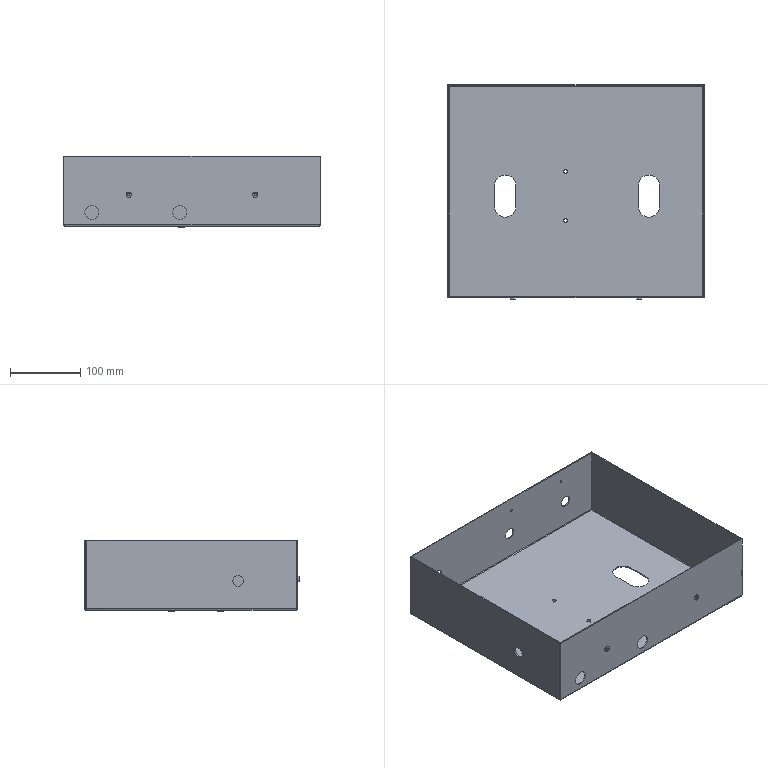Part | STEP file | air source assembly mounting plate | 1 solid | 82 faces | box 365 x 304.8 x 102 mm | volume 354021 mm3 | cylinder 44 | plane 30 | spline 8 | commonest cylinder face diameters 3.3 x8 5 x8 16 x6 2 x4 7.8 x4 8.6 x4